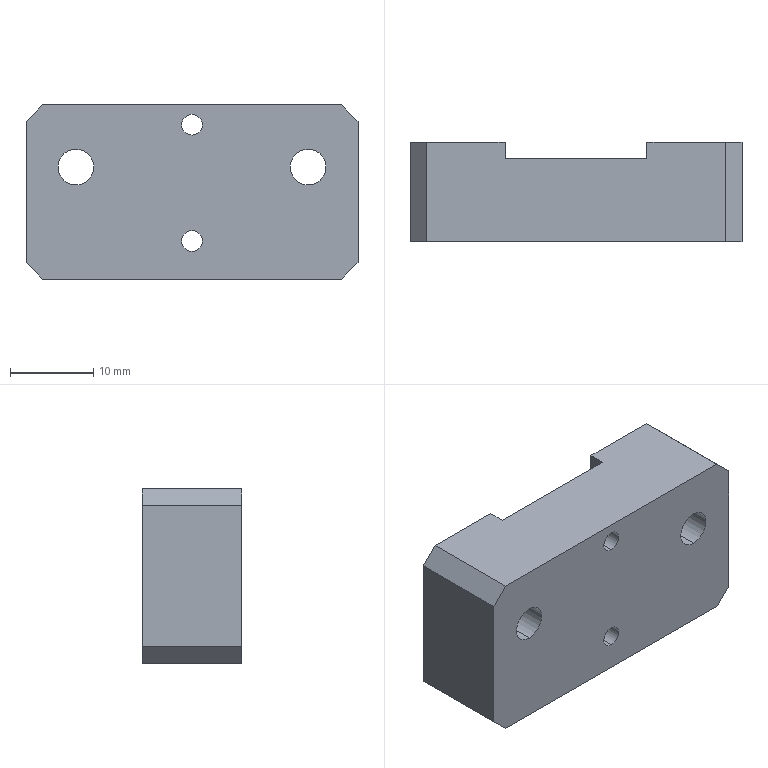Part | SolidWorks | features BaseBody 1 | 1 solid | 28 faces | box 40 x 12 x 21 mm | volume 8462 mm3 | plane 16 | cylinder 12 | commonest cylinder face diameters 2.5 x4 4.3 x4 8 x4
STEP:
#1=CARTESIAN_POINT('',(14.,7.,-1.));
#2=VERTEX_POINT('',#1);
#3=CARTESIAN_POINT('',(14.,7.,7.));
#4=VERTEX_POINT('',#3);
#5=CARTESIAN_POINT('',(14.,7.,3.));
#6=DIRECTION('',(0.,1.,0.));
#7=DIRECTION('',(0.,0.,1.));
#8=AXIS2_PLACEMENT_3D('',#5,#6,#7);
#9=CIRCLE('',#8,4.);
#10=EDGE_CURVE('',#2,#4,#9,.T.);
#11=ORIENTED_EDGE('',*,*,#10,.F.);
#12=CARTESIAN_POINT('',(14.,12.,-1.));
#13=VERTEX_POINT('',#12);
#14=CARTESIAN_POINT('',(14.,12.,-1.));
#15=DIRECTION('',(0.,1.,0.));
#16=VECTOR('',#15,1000.);
#17=LINE('',#14,#16);
#18=EDGE_CURVE('',#2,#13,#17,.T.);
#19=ORIENTED_EDGE('',*,*,#18,.T.);
#20=CARTESIAN_POINT('',(14.,12.,7.));
#21=VERTEX_POINT('',#20);
#22=CARTESIAN_POINT('',(14.,12.,3.));
#23=DIRECTION('',(0.,1.,0.));
#24=DIRECTION('',(0.,0.,1.));
#25=AXIS2_PLACEMENT_3D('',#22,#23,#24);
#26=CIRCLE('',#25,4.);
#27=EDGE_CURVE('',#13,#21,#26,.T.);
#28=ORIENTED_EDGE('',*,*,#27,.T.);
#29=CARTESIAN_POINT('',(14.,12.,7.));
#30=DIRECTION('',(0.,1.,0.));
#31=VECTOR('',#30,1000.);
#32=LINE('',#29,#31);
#33=EDGE_CURVE('',#4,#21,#32,.T.);
#34=ORIENTED_EDGE('',*,*,#33,.F.);
#35=EDGE_LOOP('',(#11,#19,#28,#34));
#36=FACE_OUTER_BOUND('',#35,.T.);
#37=CARTESIAN_POINT('',(14.,12.,3.));
#38=DIRECTION('',(0.,1.,0.));
#39=DIRECTION('',(0.,0.,1.));
#40=AXIS2_PLACEMENT_3D('',#37,#38,#39);
#41=CYLINDRICAL_SURFACE('',#40,4.);
#42=ADVANCED_FACE('',(#36),#41,.F.);
#43=CARTESIAN_POINT('',(14.,0.,0.85));
#44=VERTEX_POINT('',#43);
#45=CARTESIAN_POINT('',(14.,0.,5.15));
#46=VERTEX_POINT('',#45);
#47=CARTESIAN_POINT('',(14.,0.,3.));
#48=DIRECTION('',(0.,1.,0.));
#49=DIRECTION('',(0.,0.,1.));
#50=AXIS2_PLACEMENT_3D('',#47,#48,#49);
#51=CIRCLE('',#50,2.15);
#52=EDGE_CURVE('',#44,#46,#51,.T.);
#53=ORIENTED_EDGE('',*,*,#52,.F.);
#54=CARTESIAN_POINT('',(14.,7.,0.85));
#55=VERTEX_POINT('',#54);
#56=CARTESIAN_POINT('',(14.,12.,0.85));
#57=DIRECTION('',(0.,1.,0.));
#58=VECTOR('',#57,1000.);
#59=LINE('',#56,#58);
#60=EDGE_CURVE('',#44,#55,#59,.T.);
#61=ORIENTED_EDGE('',*,*,#60,.T.);
#62=CARTESIAN_POINT('',(14.,7.,5.15));
#63=VERTEX_POINT('',#62);
#64=CARTESIAN_POINT('',(14.,7.,3.));
#65=DIRECTION('',(0.,1.,0.));
#66=DIRECTION('',(0.,0.,1.));
#67=AXIS2_PLACEMENT_3D('',#64,#65,#66);
#68=CIRCLE('',#67,2.15);
#69=EDGE_CURVE('',#55,#63,#68,.T.);
#70=ORIENTED_EDGE('',*,*,#69,.T.);
#71=CARTESIAN_POINT('',(14.,12.,5.15));
#72=DIRECTION('',(0.,1.,0.));
#73=VECTOR('',#72,1000.);
#74=LINE('',#71,#73);
#75=EDGE_CURVE('',#46,#63,#74,.T.);
#76=ORIENTED_EDGE('',*,*,#75,.F.);
#77=EDGE_LOOP('',(#53,#61,#70,#76));
#78=FACE_OUTER_BOUND('',#77,.T.);
#79=CARTESIAN_POINT('',(14.,12.,3.));
#80=DIRECTION('',(0.,1.,0.));
#81=DIRECTION('',(0.,0.,1.));
#82=AXIS2_PLACEMENT_3D('',#79,#80,#81);
#83=CYLINDRICAL_SURFACE('',#82,2.15);
#84=ADVANCED_FACE('',(#78),#83,.F.);
#85=CARTESIAN_POINT('',(-14.,7.,-1.));
#86=VERTEX_POINT('',#85);
#87=CARTESIAN_POINT('',(-14.,7.,7.));
#88=VERTEX_POINT('',#87);
#89=CARTESIAN_POINT('',(-14.,7.,3.));
#90=DIRECTION('',(0.,1.,0.));
#91=DIRECTION('',(0.,0.,1.));
#92=AXIS2_PLACEMENT_3D('',#89,#90,#91);
#93=CIRCLE('',#92,4.);
#94=EDGE_CURVE('',#86,#88,#93,.T.);
#95=ORIENTED_EDGE('',*,*,#94,.F.);
#96=CARTESIAN_POINT('',(-14.,12.,-1.));
#97=VERTEX_POINT('',#96);
#98=CARTESIAN_POINT('',(-14.,12.,-1.));
#99=DIRECTION('',(0.,1.,0.));
#100=VECTOR('',#99,1000.);
#101=LINE('',#98,#100);
#102=EDGE_CURVE('',#86,#97,#101,.T.);
#103=ORIENTED_EDGE('',*,*,#102,.T.);
#104=CARTESIAN_POINT('',(-14.,12.,7.));
#105=VERTEX_POINT('',#104);
#106=CARTESIAN_POINT('',(-14.,12.,3.));
#107=DIRECTION('',(0.,1.,0.));
#108=DIRECTION('',(0.,0.,1.));
#109=AXIS2_PLACEMENT_3D('',#106,#107,#108);
#110=CIRCLE('',#109,4.);
#111=EDGE_CURVE('',#97,#105,#110,.T.);
#112=ORIENTED_EDGE('',*,*,#111,.T.);
#113=CARTESIAN_POINT('',(-14.,12.,7.));
#114=DIRECTION('',(0.,1.,0.));
#115=VECTOR('',#114,1000.);
#116=LINE('',#113,#115);
#117=EDGE_CURVE('',#88,#105,#116,.T.);
#118=ORIENTED_EDGE('',*,*,#117,.F.);
#119=EDGE_LOOP('',(#95,#103,#112,#118));
#120=FACE_OUTER_BOUND('',#119,.T.);
#121=CARTESIAN_POINT('',(-14.,12.,3.));
#122=DIRECTION('',(0.,1.,0.));
#123=DIRECTION('',(0.,0.,1.));
#124=AXIS2_PLACEMENT_3D('',#121,#122,#123);
#125=CYLINDRICAL_SURFACE('',#124,4.);
#126=ADVANCED_FACE('',(#120),#125,.F.);
#127=CARTESIAN_POINT('',(-14.,0.,0.85));
#128=VERTEX_POINT('',#127);
#129=CARTESIAN_POINT('',(-14.,0.,5.15));
#130=VERTEX_POINT('',#129);
#131=CARTESIAN_POINT('',(-14.,0.,3.));
#132=DIRECTION('',(0.,1.,0.));
#133=DIRECTION('',(0.,0.,1.));
#134=AXIS2_PLACEMENT_3D('',#131,#132,#133);
#135=CIRCLE('',#134,2.15);
#136=EDGE_CURVE('',#128,#130,#135,.T.);
#137=ORIENTED_EDGE('',*,*,#136,.F.);
#138=CARTESIAN_POINT('',(-14.,7.,0.85));
#139=VERTEX_POINT('',#138);
#140=CARTESIAN_POINT('',(-14.,12.,0.85));
#141=DIRECTION('',(0.,1.,0.));
#142=VECTOR('',#141,1000.);
#143=LINE('',#140,#142);
#144=EDGE_CURVE('',#128,#139,#143,.T.);
#145=ORIENTED_EDGE('',*,*,#144,.T.);
#146=CARTESIAN_POINT('',(-14.,7.,5.15));
#147=VERTEX_POINT('',#146);
#148=CARTESIAN_POINT('',(-14.,7.,3.));
#149=DIRECTION('',(0.,1.,0.));
#150=DIRECTION('',(0.,0.,1.));
#151=AXIS2_PLACEMENT_3D('',#148,#149,#150);
#152=CIRCLE('',#151,2.15);
#153=EDGE_CURVE('',#139,#147,#152,.T.);
#154=ORIENTED_EDGE('',*,*,#153,.T.);
#155=CARTESIAN_POINT('',(-14.,12.,5.15));
#156=DIRECTION('',(0.,1.,0.));
#157=VECTOR('',#156,1000.);
#158=LINE('',#155,#157);
#159=EDGE_CURVE('',#130,#147,#158,.T.);
#160=ORIENTED_EDGE('',*,*,#159,.F.);
#161=EDGE_LOOP('',(#137,#145,#154,#160));
#162=FACE_OUTER_BOUND('',#161,.T.);
#163=CARTESIAN_POINT('',(-14.,12.,3.));
#164=DIRECTION('',(0.,1.,0.));
#165=DIRECTION('',(0.,0.,1.));
#166=AXIS2_PLACEMENT_3D('',#163,#164,#165);
#167=CYLINDRICAL_SURFACE('',#166,2.15);
#168=ADVANCED_FACE('',(#162),#167,.F.);
#169=CARTESIAN_POINT('',(0.,0.,6.85));
#170=VERTEX_POINT('',#169);
#171=CARTESIAN_POINT('',(0.,0.,9.35));
#172=VERTEX_POINT('',#171);
#173=CARTESIAN_POINT('',(0.,0.,8.1));
#174=DIRECTION('',(0.,1.,0.));
#175=DIRECTION('',(0.,0.,1.));
#176=AXIS2_PLACEMENT_3D('',#173,#174,#175);
#177=CIRCLE('',#176,1.25);
#178=EDGE_CURVE('',#170,#172,#177,.T.);
#179=ORIENTED_EDGE('',*,*,#178,.F.);
#180=CARTESIAN_POINT('',(0.,10.,6.85));
#181=VERTEX_POINT('',#180);
#182=CARTESIAN_POINT('',(0.,12.,6.85));
#183=DIRECTION('',(0.,1.,0.));
#184=VECTOR('',#183,1000.);
#185=LINE('',#182,#184);
#186=EDGE_CURVE('',#170,#181,#185,.T.);
#187=ORIENTED_EDGE('',*,*,#186,.T.);
#188=CARTESIAN_POINT('',(0.,10.,9.35));
#189=VERTEX_POINT('',#188);
#190=CARTESIAN_POINT('',(0.,10.,8.1));
#191=DIRECTION('',(0.,1.,0.));
#192=DIRECTION('',(0.,0.,1.));
#193=AXIS2_PLACEMENT_3D('',#190,#191,#192);
#194=CIRCLE('',#193,1.25);
#195=EDGE_CURVE('',#181,#189,#194,.T.);
#196=ORIENTED_EDGE('',*,*,#195,.T.);
#197=CARTESIAN_POINT('',(0.,12.,9.35));
#198=DIRECTION('',(0.,1.,0.));
#199=VECTOR('',#198,1000.);
#200=LINE('',#197,#199);
#201=EDGE_CURVE('',#172,#189,#200,.T.);
#202=ORIENTED_EDGE('',*,*,#201,.F.);
#203=EDGE_LOOP('',(#179,#187,#196,#202));
#204=FACE_OUTER_BOUND('',#203,.T.);
#205=CARTESIAN_POINT('',(0.,12.,8.1));
#206=DIRECTION('',(0.,1.,0.));
#207=DIRECTION('',(0.,0.,1.));
#208=AXIS2_PLACEMENT_3D('',#205,#206,#207);
#209=CYLINDRICAL_SURFACE('',#208,1.25);
#210=ADVANCED_FACE('',(#204),#209,.F.);
#211=CARTESIAN_POINT('',(0.,0.,-7.15));
#212=VERTEX_POINT('',#211);
#213=CARTESIAN_POINT('',(0.,0.,-4.65));
#214=VERTEX_POINT('',#213);
#215=CARTESIAN_POINT('',(0.,0.,-5.9));
#216=DIRECTION('',(0.,1.,0.));
#217=DIRECTION('',(0.,0.,1.));
#218=AXIS2_PLACEMENT_3D('',#215,#216,#217);
#219=CIRCLE('',#218,1.25);
#220=EDGE_CURVE('',#212,#214,#219,.T.);
#221=ORIENTED_EDGE('',*,*,#220,.F.);
#222=CARTESIAN_POINT('',(0.,10.,-7.15));
#223=VERTEX_POINT('',#222);
#224=CARTESIAN_POINT('',(0.,12.,-7.15));
#225=DIRECTION('',(0.,1.,0.));
#226=VECTOR('',#225,1000.);
#227=LINE('',#224,#226);
#228=EDGE_CURVE('',#212,#223,#227,.T.);
#229=ORIENTED_EDGE('',*,*,#228,.T.);
#230=CARTESIAN_POINT('',(0.,10.,-4.65));
#231=VERTEX_POINT('',#230);
#232=CARTESIAN_POINT('',(0.,10.,-5.9));
#233=DIRECTION('',(0.,1.,0.));
#234=DIRECTION('',(0.,0.,1.));
#235=AXIS2_PLACEMENT_3D('',#232,#233,#234);
#236=CIRCLE('',#235,1.25);
#237=EDGE_CURVE('',#223,#231,#236,.T.);
#238=ORIENTED_EDGE('',*,*,#237,.T.);
#239=CARTESIAN_POINT('',(0.,12.,-4.65));
#240=DIRECTION('',(0.,1.,0.));
#241=VECTOR('',#240,1000.);
#242=LINE('',#239,#241);
#243=EDGE_CURVE('',#214,#231,#242,.T.);
#244=ORIENTED_EDGE('',*,*,#243,.F.);
#245=EDGE_LOOP('',(#221,#229,#238,#244));
#246=FACE_OUTER_BOUND('',#245,.T.);
#247=CARTESIAN_POINT('',(0.,12.,-5.9));
#248=DIRECTION('',(0.,1.,0.));
#249=DIRECTION('',(0.,0.,1.));
#250=AXIS2_PLACEMENT_3D('',#247,#248,#249);
#251=CYLINDRICAL_SURFACE('',#250,1.25);
#252=ADVANCED_FACE('',(#246),#251,.F.);
#253=CARTESIAN_POINT('',(-20.,12.,8.5));
#254=VERTEX_POINT('',#253);
#255=CARTESIAN_POINT('',(-18.,12.,10.5));
#256=VERTEX_POINT('',#255);
#257=CARTESIAN_POINT('',(-14.25,12.,14.25));
#258=DIRECTION('',(0.7071,0.,0.7071));
#259=VECTOR('',#258,1000.);
#260=LINE('',#257,#259);
#261=EDGE_CURVE('',#254,#256,#260,.T.);
#262=ORIENTED_EDGE('',*,*,#261,.F.);
#263=CARTESIAN_POINT('',(-20.,0.,8.5));
#264=VERTEX_POINT('',#263);
#265=CARTESIAN_POINT('',(-20.,12.,8.5));
#266=DIRECTION('',(0.,1.,0.));
#267=VECTOR('',#266,1000.);
#268=LINE('',#265,#267);
#269=EDGE_CURVE('',#264,#254,#268,.T.);
#270=ORIENTED_EDGE('',*,*,#269,.F.);
#271=CARTESIAN_POINT('',(-18.,0.,10.5));
#272=VERTEX_POINT('',#271);
#273=CARTESIAN_POINT('',(-18.,0.,10.5));
#274=DIRECTION('',(-0.7071,0.,-0.7071));
#275=VECTOR('',#274,1000.);
#276=LINE('',#273,#275);
#277=EDGE_CURVE('',#272,#264,#276,.T.);
#278=ORIENTED_EDGE('',*,*,#277,.F.);
#279=CARTESIAN_POINT('',(-18.,12.,10.5));
#280=DIRECTION('',(0.,-1.,0.));
#281=VECTOR('',#280,1000.);
#282=LINE('',#279,#281);
#283=EDGE_CURVE('',#256,#272,#282,.T.);
#284=ORIENTED_EDGE('',*,*,#283,.F.);
#285=EDGE_LOOP('',(#262,#270,#278,#284));
#286=FACE_OUTER_BOUND('',#285,.T.);
#287=CARTESIAN_POINT('',(-18.,12.,10.5));
#288=DIRECTION('',(0.7071,0.,-0.7071));
#289=DIRECTION('',(0.,-1.,0.));
#290=AXIS2_PLACEMENT_3D('',#287,#288,#289);
#291=PLANE('',#290);
#292=ADVANCED_FACE('',(#286),#291,.F.);
#293=CARTESIAN_POINT('',(18.,12.,10.5));
#294=VERTEX_POINT('',#293);
#295=CARTESIAN_POINT('',(20.,12.,8.5));
#296=VERTEX_POINT('',#295);
#297=CARTESIAN_POINT('',(14.25,12.,14.25));
#298=DIRECTION('',(0.7071,0.,-0.7071));
#299=VECTOR('',#298,1000.);
#300=LINE('',#297,#299);
#301=EDGE_CURVE('',#294,#296,#300,.T.);
#302=ORIENTED_EDGE('',*,*,#301,.F.);
#303=CARTESIAN_POINT('',(18.,0.,10.5));
#304=VERTEX_POINT('',#303);
#305=CARTESIAN_POINT('',(18.,12.,10.5));
#306=DIRECTION('',(0.,1.,0.));
#307=VECTOR('',#306,1000.);
#308=LINE('',#305,#307);
#309=EDGE_CURVE('',#304,#294,#308,.T.);
#310=ORIENTED_EDGE('',*,*,#309,.F.);
#311=CARTESIAN_POINT('',(20.,0.,8.5));
#312=VERTEX_POINT('',#311);
#313=CARTESIAN_POINT('',(20.,0.,8.5));
#314=DIRECTION('',(-0.7071,0.,0.7071));
#315=VECTOR('',#314,1000.);
#316=LINE('',#313,#315);
#317=EDGE_CURVE('',#312,#304,#316,.T.);
#318=ORIENTED_EDGE('',*,*,#317,.F.);
#319=CARTESIAN_POINT('',(20.,12.,8.5));
#320=DIRECTION('',(0.,-1.,0.));
#321=VECTOR('',#320,1000.);
#322=LINE('',#319,#321);
#323=EDGE_CURVE('',#296,#312,#322,.T.);
#324=ORIENTED_EDGE('',*,*,#323,.F.);
#325=EDGE_LOOP('',(#302,#310,#318,#324));
#326=FACE_OUTER_BOUND('',#325,.T.);
#327=CARTESIAN_POINT('',(20.,12.,8.5));
#328=DIRECTION('',(-0.7071,0.,-0.7071));
#329=DIRECTION('',(-0.7071,0.,0.7071));
#330=AXIS2_PLACEMENT_3D('',#327,#328,#329);
#331=PLANE('',#330);
#332=ADVANCED_FACE('',(#326),#331,.F.);
#333=CARTESIAN_POINT('',(20.,12.,-8.5));
#334=VERTEX_POINT('',#333);
#335=CARTESIAN_POINT('',(18.,12.,-10.5));
#336=VERTEX_POINT('',#335);
#337=CARTESIAN_POINT('',(14.25,12.,-14.25));
#338=DIRECTION('',(-0.7071,0.,-0.7071));
#339=VECTOR('',#338,1000.);
#340=LINE('',#337,#339);
#341=EDGE_CURVE('',#334,#336,#340,.T.);
#342=ORIENTED_EDGE('',*,*,#341,.F.);
#343=CARTESIAN_POINT('',(20.,0.,-8.5));
#344=VERTEX_POINT('',#343);
#345=CARTESIAN_POINT('',(20.,12.,-8.5));
#346=DIRECTION('',(0.,1.,0.));
#347=VECTOR('',#346,1000.);
#348=LINE('',#345,#347);
#349=EDGE_CURVE('',#344,#334,#348,.T.);
#350=ORIENTED_EDGE('',*,*,#349,.F.);
#351=CARTESIAN_POINT('',(18.,0.,-10.5));
#352=VERTEX_POINT('',#351);
#353=CARTESIAN_POINT('',(18.,0.,-10.5));
#354=DIRECTION('',(0.7071,0.,0.7071));
#355=VECTOR('',#354,1000.);
#356=LINE('',#353,#355);
#357=EDGE_CURVE('',#352,#344,#356,.T.);
#358=ORIENTED_EDGE('',*,*,#357,.F.);
#359=CARTESIAN_POINT('',(18.,12.,-10.5));
#360=DIRECTION('',(0.,-1.,0.));
#361=VECTOR('',#360,1000.);
#362=LINE('',#359,#361);
#363=EDGE_CURVE('',#336,#352,#362,.T.);
#364=ORIENTED_EDGE('',*,*,#363,.F.);
#365=EDGE_LOOP('',(#342,#350,#358,#364));
#366=FACE_OUTER_BOUND('',#365,.T.);
#367=CARTESIAN_POINT('',(18.,12.,-10.5));
#368=DIRECTION('',(-0.7071,0.,0.7071));
#369=DIRECTION('',(0.,1.,0.));
#370=AXIS2_PLACEMENT_3D('',#367,#368,#369);
#371=PLANE('',#370);
#372=ADVANCED_FACE('',(#366),#371,.F.);
#373=CARTESIAN_POINT('',(-18.,12.,-10.5));
#374=VERTEX_POINT('',#373);
#375=CARTESIAN_POINT('',(-20.,12.,-8.5));
#376=VERTEX_POINT('',#375);
#377=CARTESIAN_POINT('',(-14.25,12.,-14.25));
#378=DIRECTION('',(-0.7071,0.,0.7071));
#379=VECTOR('',#378,1000.);
#380=LINE('',#377,#379);
#381=EDGE_CURVE('',#374,#376,#380,.T.);
#382=ORIENTED_EDGE('',*,*,#381,.F.);
#383=CARTESIAN_POINT('',(-18.,0.,-10.5));
#384=VERTEX_POINT('',#383);
#385=CARTESIAN_POINT('',(-18.,12.,-10.5));
#386=DIRECTION('',(0.,1.,0.));
#387=VECTOR('',#386,1000.);
#388=LINE('',#385,#387);
#389=EDGE_CURVE('',#384,#374,#388,.T.);
#390=ORIENTED_EDGE('',*,*,#389,.F.);
#391=CARTESIAN_POINT('',(-20.,0.,-8.5));
#392=VERTEX_POINT('',#391);
#393=CARTESIAN_POINT('',(-20.,0.,-8.5));
#394=DIRECTION('',(0.7071,0.,-0.7071));
#395=VECTOR('',#394,1000.);
#396=LINE('',#393,#395);
#397=EDGE_CURVE('',#392,#384,#396,.T.);
#398=ORIENTED_EDGE('',*,*,#397,.F.);
#399=CARTESIAN_POINT('',(-20.,12.,-8.5));
#400=DIRECTION('',(0.,-1.,0.));
#401=VECTOR('',#400,1000.);
#402=LINE('',#399,#401);
#403=EDGE_CURVE('',#376,#392,#402,.T.);
#404=ORIENTED_EDGE('',*,*,#403,.F.);
#405=EDGE_LOOP('',(#382,#390,#398,#404));
#406=FACE_OUTER_BOUND('',#405,.T.);
#407=CARTESIAN_POINT('',(-20.,12.,-8.5));
#408=DIRECTION('',(0.7071,0.,0.7071));
#409=DIRECTION('',(0.,-1.,0.));
#410=AXIS2_PLACEMENT_3D('',#407,#408,#409);
#411=PLANE('',#410);
#412=ADVANCED_FACE('',(#406),#411,.F.);
#413=CARTESIAN_POINT('',(14.,7.,3.));
#414=DIRECTION('',(0.,1.,0.));
#415=DIRECTION('',(0.,0.,1.));
#416=AXIS2_PLACEMENT_3D('',#413,#414,#415);
#417=CIRCLE('',#416,2.15);
#418=EDGE_CURVE('',#63,#55,#417,.T.);
#419=ORIENTED_EDGE('',*,*,#418,.F.);
#420=ORIENTED_EDGE('',*,*,#69,.F.);
#421=EDGE_LOOP('',(#419,#420));
#422=FACE_BOUND('',#421,.T.);
#423=CARTESIAN_POINT('',(14.,7.,3.));
#424=DIRECTION('',(0.,1.,0.));
#425=DIRECTION('',(0.,0.,1.));
#426=AXIS2_PLACEMENT_3D('',#423,#424,#425);
#427=CIRCLE('',#426,4.);
#428=EDGE_CURVE('',#4,#2,#427,.T.);
#429=ORIENTED_EDGE('',*,*,#428,.T.);
#430=ORIENTED_EDGE('',*,*,#10,.T.);
#431=EDGE_LOOP('',(#429,#430));
#432=FACE_OUTER_BOUND('',#431,.T.);
#433=CARTESIAN_POINT('',(16.15,7.,3.));
#434=DIRECTION('',(0.,-1.,0.));
#435=DIRECTION('',(0.,0.,-1.));
#436=AXIS2_PLACEMENT_3D('',#433,#434,#435);
#437=PLANE('',#436);
#438=ADVANCED_FACE('',(#422,#432),#437,.F.);
#439=CARTESIAN_POINT('',(-14.,7.,3.));
#440=DIRECTION('',(0.,1.,0.));
#441=DIRECTION('',(0.,0.,1.));
#442=AXIS2_PLACEMENT_3D('',#439,#440,#441);
#443=CIRCLE('',#442,2.15);
#444=EDGE_CURVE('',#147,#139,#443,.T.);
#445=ORIENTED_EDGE('',*,*,#444,.F.);
#446=ORIENTED_EDGE('',*,*,#153,.F.);
#447=EDGE_LOOP('',(#445,#446));
#448=FACE_BOUND('',#447,.T.);
#449=CARTESIAN_POINT('',(-14.,7.,3.));
#450=DIRECTION('',(0.,1.,0.));
#451=DIRECTION('',(0.,0.,1.));
#452=AXIS2_PLACEMENT_3D('',#449,#450,#451);
#453=CIRCLE('',#452,4.);
#454=EDGE_CURVE('',#88,#86,#453,.T.);
#455=ORIENTED_EDGE('',*,*,#454,.T.);
#456=ORIENTED_EDGE('',*,*,#94,.T.);
#457=EDGE_LOOP('',(#455,#456));
#458=FACE_OUTER_BOUND('',#457,.T.);
#459=CARTESIAN_POINT('',(-11.85,7.,3.));
#460=DIRECTION('',(0.,-1.,0.));
#461=DIRECTION('',(0.,0.,-1.));
#462=AXIS2_PLACEMENT_3D('',#459,#460,#461);
#463=PLANE('',#462);
#464=ADVANCED_FACE('',(#448,#458),#463,.F.);
#465=CARTESIAN_POINT('',(-8.55,12.,-10.5));
#466=VERTEX_POINT('',#465);
#467=CARTESIAN_POINT('',(-8.55,12.,10.5));
#468=VERTEX_POINT('',#467);
#469=CARTESIAN_POINT('',(-8.55,12.,0.));
#470=DIRECTION('',(0.,0.,1.));
#471=VECTOR('',#470,1000.);
#472=LINE('',#469,#471);
#473=EDGE_CURVE('',#466,#468,#472,.T.);
#474=ORIENTED_EDGE('',*,*,#473,.T.);
#475=CARTESIAN_POINT('',(-8.55,10.,10.5));
#476=VERTEX_POINT('',#475);
#477=CARTESIAN_POINT('',(-8.55,12.,10.5));
#478=DIRECTION('',(0.,1.,0.));
#479=VECTOR('',#478,1000.);
#480=LINE('',#477,#479);
#481=EDGE_CURVE('',#476,#468,#480,.T.);
#482=ORIENTED_EDGE('',*,*,#481,.F.);
#483=CARTESIAN_POINT('',(-8.55,10.,-10.5));
#484=VERTEX_POINT('',#483);
#485=CARTESIAN_POINT('',(-8.55,10.,-15.));
#486=DIRECTION('',(0.,0.,1.));
#487=VECTOR('',#486,1000.);
#488=LINE('',#485,#487);
#489=EDGE_CURVE('',#484,#476,#488,.T.);
#490=ORIENTED_EDGE('',*,*,#489,.F.);
#491=CARTESIAN_POINT('',(-8.55,12.,-10.5));
#492=DIRECTION('',(0.,-1.,0.));
#493=VECTOR('',#492,1000.);
#494=LINE('',#491,#493);
#495=EDGE_CURVE('',#466,#484,#494,.T.);
#496=ORIENTED_EDGE('',*,*,#495,.F.);
#497=EDGE_LOOP('',(#474,#482,#490,#496));
#498=FACE_OUTER_BOUND('',#497,.T.);
#499=CARTESIAN_POINT('',(-8.55,10.,-15.));
#500=DIRECTION('',(-1.,0.,0.));
#501=DIRECTION('',(0.,1.,0.));
#502=AXIS2_PLACEMENT_3D('',#499,#500,#501);
#503=PLANE('',#502);
#504=ADVANCED_FACE('',(#498),#503,.F.);
#505=CARTESIAN_POINT('',(8.55,10.,10.5));
#506=VERTEX_POINT('',#505);
#507=CARTESIAN_POINT('',(8.55,10.,-10.5));
#508=VERTEX_POINT('',#507);
#509=CARTESIAN_POINT('',(8.55,10.,-15.));
#510=DIRECTION('',(0.,0.,-1.));
#511=VECTOR('',#510,1000.);
#512=LINE('',#509,#511);
#513=EDGE_CURVE('',#506,#508,#512,.T.);
#514=ORIENTED_EDGE('',*,*,#513,.F.);
#515=CARTESIAN_POINT('',(8.55,12.,10.5));
#516=VERTEX_POINT('',#515);
#517=CARTESIAN_POINT('',(8.55,12.,10.5));
#518=DIRECTION('',(0.,-1.,0.));
#519=VECTOR('',#518,1000.);
#520=LINE('',#517,#519);
#521=EDGE_CURVE('',#516,#506,#520,.T.);
#522=ORIENTED_EDGE('',*,*,#521,.F.);
#523=CARTESIAN_POINT('',(8.55,12.,-10.5));
#524=VERTEX_POINT('',#523);
#525=CARTESIAN_POINT('',(8.55,12.,0.));
#526=DIRECTION('',(0.,0.,-1.));
#527=VECTOR('',#526,1000.);
#528=LINE('',#525,#527);
#529=EDGE_CURVE('',#516,#524,#528,.T.);
#530=ORIENTED_EDGE('',*,*,#529,.T.);
#531=CARTESIAN_POINT('',(8.55,12.,-10.5));
#532=DIRECTION('',(0.,1.,0.));
#533=VECTOR('',#532,1000.);
#534=LINE('',#531,#533);
#535=EDGE_CURVE('',#508,#524,#534,.T.);
#536=ORIENTED_EDGE('',*,*,#535,.F.);
#537=EDGE_LOOP('',(#514,#522,#530,#536));
#538=FACE_OUTER_BOUND('',#537,.T.);
#539=CARTESIAN_POINT('',(8.55,10.,-15.));
#540=DIRECTION('',(1.,0.,0.));
#541=DIRECTION('',(0.,0.,-1.));
#542=AXIS2_PLACEMENT_3D('',#539,#540,#541);
#543=PLANE('',#542);
#544=ADVANCED_FACE('',(#538),#543,.F.);
#545=CARTESIAN_POINT('',(0.,10.,-5.9));
#546=DIRECTION('',(0.,1.,0.));
#547=DIRECTION('',(0.,0.,1.));
#548=AXIS2_PLACEMENT_3D('',#545,#546,#547);
#549=CIRCLE('',#548,1.25);
#550=EDGE_CURVE('',#231,#223,#549,.T.);
#551=ORIENTED_EDGE('',*,*,#550,.F.);
#552=ORIENTED_EDGE('',*,*,#237,.F.);
#553=EDGE_LOOP('',(#551,#552));
#554=FACE_BOUND('',#553,.T.);
#555=CARTESIAN_POINT('',(0.,10.,8.1));
#556=DIRECTION('',(0.,1.,0.));
#557=DIRECTION('',(0.,0.,1.));
#558=AXIS2_PLACEMENT_3D('',#555,#556,#557);
#559=CIRCLE('',#558,1.25);
#560=EDGE_CURVE('',#189,#181,#559,.T.);
#561=ORIENTED_EDGE('',*,*,#560,.F.);
#562=ORIENTED_EDGE('',*,*,#195,.F.);
#563=EDGE_LOOP('',(#561,#562));
#564=FACE_BOUND('',#563,.T.);
#565=CARTESIAN_POINT('',(-20.,10.,-10.5));
#566=DIRECTION('',(-1.,0.,0.));
#567=VECTOR('',#566,1000.);
#568=LINE('',#565,#567);
#569=EDGE_CURVE('',#508,#484,#568,.T.);
#570=ORIENTED_EDGE('',*,*,#569,.T.);
#571=ORIENTED_EDGE('',*,*,#489,.T.);
#572=CARTESIAN_POINT('',(-20.,10.,10.5));
#573=DIRECTION('',(1.,0.,0.));
#574=VECTOR('',#573,1000.);
#575=LINE('',#572,#574);
#576=EDGE_CURVE('',#476,#506,#575,.T.);
#577=ORIENTED_EDGE('',*,*,#576,.T.);
#578=ORIENTED_EDGE('',*,*,#513,.T.);
#579=EDGE_LOOP('',(#570,#571,#577,#578));
#580=FACE_OUTER_BOUND('',#579,.T.);
#581=CARTESIAN_POINT('',(0.,10.,0.));
#582=DIRECTION('',(0.,1.,0.));
#583=DIRECTION('',(1.,0.,0.));
#584=AXIS2_PLACEMENT_3D('',#581,#582,#583);
#585=PLANE('',#584);
#586=ADVANCED_FACE('',(#554,#564,#580),#585,.T.);
#587=CARTESIAN_POINT('',(0.,0.,-5.9));
#588=DIRECTION('',(0.,1.,0.));
#589=DIRECTION('',(0.,0.,1.));
#590=AXIS2_PLACEMENT_3D('',#587,#588,#589);
#591=CIRCLE('',#590,1.25);
#592=EDGE_CURVE('',#214,#212,#591,.T.);
#593=ORIENTED_EDGE('',*,*,#592,.T.);
#594=ORIENTED_EDGE('',*,*,#220,.T.);
#595=EDGE_LOOP('',(#593,#594));
#596=FACE_BOUND('',#595,.T.);
#597=CARTESIAN_POINT('',(0.,0.,8.1));
#598=DIRECTION('',(0.,1.,0.));
#599=DIRECTION('',(0.,0.,1.));
#600=AXIS2_PLACEMENT_3D('',#597,#598,#599);
#601=CIRCLE('',#600,1.25);
#602=EDGE_CURVE('',#172,#170,#601,.T.);
#603=ORIENTED_EDGE('',*,*,#602,.T.);
#604=ORIENTED_EDGE('',*,*,#178,.T.);
#605=EDGE_LOOP('',(#603,#604));
#606=FACE_BOUND('',#605,.T.);
#607=CARTESIAN_POINT('',(-14.,0.,3.));
#608=DIRECTION('',(0.,1.,0.));
#609=DIRECTION('',(0.,0.,1.));
#610=AXIS2_PLACEMENT_3D('',#607,#608,#609);
#611=CIRCLE('',#610,2.15);
#612=EDGE_CURVE('',#130,#128,#611,.T.);
#613=ORIENTED_EDGE('',*,*,#612,.T.);
#614=ORIENTED_EDGE('',*,*,#136,.T.);
#615=EDGE_LOOP('',(#613,#614));
#616=FACE_BOUND('',#615,.T.);
#617=CARTESIAN_POINT('',(14.,0.,3.));
#618=DIRECTION('',(0.,1.,0.));
#619=DIRECTION('',(0.,0.,1.));
#620=AXIS2_PLACEMENT_3D('',#617,#618,#619);
#621=CIRCLE('',#620,2.15);
#622=EDGE_CURVE('',#46,#44,#621,.T.);
#623=ORIENTED_EDGE('',*,*,#622,.T.);
#624=ORIENTED_EDGE('',*,*,#52,.T.);
#625=EDGE_LOOP('',(#623,#624));
#626=FACE_BOUND('',#625,.T.);
#627=CARTESIAN_POINT('',(-20.,0.,-10.5));
#628=DIRECTION('',(0.,0.,1.));
#629=VECTOR('',#628,1000.);
#630=LINE('',#627,#629);
#631=EDGE_CURVE('',#392,#264,#630,.T.);
#632=ORIENTED_EDGE('',*,*,#631,.F.);
#633=ORIENTED_EDGE('',*,*,#397,.T.);
#634=CARTESIAN_POINT('',(-20.,0.,-10.5));
#635=DIRECTION('',(-1.,0.,0.));
#636=VECTOR('',#635,1000.);
#637=LINE('',#634,#636);
#638=EDGE_CURVE('',#352,#384,#637,.T.);
#639=ORIENTED_EDGE('',*,*,#638,.F.);
#640=ORIENTED_EDGE('',*,*,#357,.T.);
#641=CARTESIAN_POINT('',(20.,0.,-10.5));
#642=DIRECTION('',(0.,0.,-1.));
#643=VECTOR('',#642,1000.);
#644=LINE('',#641,#643);
#645=EDGE_CURVE('',#312,#344,#644,.T.);
#646=ORIENTED_EDGE('',*,*,#645,.F.);
#647=ORIENTED_EDGE('',*,*,#317,.T.);
#648=CARTESIAN_POINT('',(-20.,0.,10.5));
#649=DIRECTION('',(1.,0.,0.));
#650=VECTOR('',#649,1000.);
#651=LINE('',#648,#650);
#652=EDGE_CURVE('',#272,#304,#651,.T.);
#653=ORIENTED_EDGE('',*,*,#652,.F.);
#654=ORIENTED_EDGE('',*,*,#277,.T.);
#655=EDGE_LOOP('',(#632,#633,#639,#640,#646,#647,#653,#654));
#656=FACE_OUTER_BOUND('',#655,.T.);
#657=CARTESIAN_POINT('',(0.,0.,0.));
#658=DIRECTION('',(0.,1.,0.));
#659=DIRECTION('',(1.,0.,0.));
#660=AXIS2_PLACEMENT_3D('',#657,#658,#659);
#661=PLANE('',#660);
#662=ADVANCED_FACE('',(#596,#606,#616,#626,#656),#661,.F.);
#663=CARTESIAN_POINT('',(-14.,12.,3.));
#664=DIRECTION('',(0.,1.,0.));
#665=DIRECTION('',(0.,0.,1.));
#666=AXIS2_PLACEMENT_3D('',#663,#664,#665);
#667=CIRCLE('',#666,4.);
#668=EDGE_CURVE('',#105,#97,#667,.T.);
#669=ORIENTED_EDGE('',*,*,#668,.F.);
#670=ORIENTED_EDGE('',*,*,#111,.F.);
#671=EDGE_LOOP('',(#669,#670));
#672=FACE_BOUND('',#671,.T.);
#673=CARTESIAN_POINT('',(-20.,12.,-10.5));
#674=DIRECTION('',(-1.,0.,0.));
#675=VECTOR('',#674,1000.);
#676=LINE('',#673,#675);
#677=EDGE_CURVE('',#466,#374,#676,.T.);
#678=ORIENTED_EDGE('',*,*,#677,.T.);
#679=ORIENTED_EDGE('',*,*,#381,.T.);
#680=CARTESIAN_POINT('',(-20.,12.,-10.5));
#681=DIRECTION('',(0.,0.,1.));
#682=VECTOR('',#681,1000.);
#683=LINE('',#680,#682);
#684=EDGE_CURVE('',#376,#254,#683,.T.);
#685=ORIENTED_EDGE('',*,*,#684,.T.);
#686=ORIENTED_EDGE('',*,*,#261,.T.);
#687=CARTESIAN_POINT('',(-20.,12.,10.5));
#688=DIRECTION('',(1.,0.,0.));
#689=VECTOR('',#688,1000.);
#690=LINE('',#687,#689);
#691=EDGE_CURVE('',#256,#468,#690,.T.);
#692=ORIENTED_EDGE('',*,*,#691,.T.);
#693=ORIENTED_EDGE('',*,*,#473,.F.);
#694=EDGE_LOOP('',(#678,#679,#685,#686,#692,#693));
#695=FACE_OUTER_BOUND('',#694,.T.);
#696=CARTESIAN_POINT('',(0.,12.,0.));
#697=DIRECTION('',(0.,1.,0.));
#698=DIRECTION('',(1.,0.,0.));
#699=AXIS2_PLACEMENT_3D('',#696,#697,#698);
#700=PLANE('',#699);
#701=ADVANCED_FACE('',(#672,#695),#700,.T.);
#702=ORIENTED_EDGE('',*,*,#652,.T.);
#703=ORIENTED_EDGE('',*,*,#309,.T.);
#704=CARTESIAN_POINT('',(-20.,12.,10.5));
#705=DIRECTION('',(1.,0.,0.));
#706=VECTOR('',#705,1000.);
#707=LINE('',#704,#706);
#708=EDGE_CURVE('',#516,#294,#707,.T.);
#709=ORIENTED_EDGE('',*,*,#708,.F.);
#710=ORIENTED_EDGE('',*,*,#521,.T.);
#711=ORIENTED_EDGE('',*,*,#576,.F.);
#712=ORIENTED_EDGE('',*,*,#481,.T.);
#713=ORIENTED_EDGE('',*,*,#691,.F.);
#714=ORIENTED_EDGE('',*,*,#283,.T.);
#715=EDGE_LOOP('',(#702,#703,#709,#710,#711,#712,#713,#714));
#716=FACE_OUTER_BOUND('',#715,.T.);
#717=CARTESIAN_POINT('',(-20.,12.,10.5));
#718=DIRECTION('',(0.,0.,-1.));
#719=DIRECTION('',(0.,-1.,0.));
#720=AXIS2_PLACEMENT_3D('',#717,#718,#719);
#721=PLANE('',#720);
#722=ADVANCED_FACE('',(#716),#721,.F.);
#723=ORIENTED_EDGE('',*,*,#684,.F.);
#724=ORIENTED_EDGE('',*,*,#403,.T.);
#725=ORIENTED_EDGE('',*,*,#631,.T.);
#726=ORIENTED_EDGE('',*,*,#269,.T.);
#727=EDGE_LOOP('',(#723,#724,#725,#726));
#728=FACE_OUTER_BOUND('',#727,.T.);
#729=CARTESIAN_POINT('',(-20.,12.,-10.5));
#730=DIRECTION('',(1.,0.,0.));
#731=DIRECTION('',(0.,0.,-1.));
#732=AXIS2_PLACEMENT_3D('',#729,#730,#731);
#733=PLANE('',#732);
#734=ADVANCED_FACE('',(#728),#733,.F.);
#735=ORIENTED_EDGE('',*,*,#638,.T.);
#736=ORIENTED_EDGE('',*,*,#389,.T.);
#737=ORIENTED_EDGE('',*,*,#677,.F.);
#738=ORIENTED_EDGE('',*,*,#495,.T.);
#739=ORIENTED_EDGE('',*,*,#569,.F.);
#740=ORIENTED_EDGE('',*,*,#535,.T.);
#741=CARTESIAN_POINT('',(-20.,12.,-10.5));
#742=DIRECTION('',(-1.,0.,0.));
#743=VECTOR('',#742,1000.);
#744=LINE('',#741,#743);
#745=EDGE_CURVE('',#336,#524,#744,.T.);
#746=ORIENTED_EDGE('',*,*,#745,.F.);
#747=ORIENTED_EDGE('',*,*,#363,.T.);
#748=EDGE_LOOP('',(#735,#736,#737,#738,#739,#740,#746,#747));
#749=FACE_OUTER_BOUND('',#748,.T.);
#750=CARTESIAN_POINT('',(-20.,12.,-10.5));
#751=DIRECTION('',(0.,0.,1.));
#752=DIRECTION('',(1.,0.,0.));
#753=AXIS2_PLACEMENT_3D('',#750,#751,#752);
#754=PLANE('',#753);
#755=ADVANCED_FACE('',(#749),#754,.F.);
#756=ORIENTED_EDGE('',*,*,#645,.T.);
#757=ORIENTED_EDGE('',*,*,#349,.T.);
#758=CARTESIAN_POINT('',(20.,12.,-10.5));
#759=DIRECTION('',(0.,0.,-1.));
#760=VECTOR('',#759,1000.);
#761=LINE('',#758,#760);
#762=EDGE_CURVE('',#296,#334,#761,.T.);
#763=ORIENTED_EDGE('',*,*,#762,.F.);
#764=ORIENTED_EDGE('',*,*,#323,.T.);
#765=EDGE_LOOP('',(#756,#757,#763,#764));
#766=FACE_OUTER_BOUND('',#765,.T.);
#767=CARTESIAN_POINT('',(20.,12.,-10.5));
#768=DIRECTION('',(-1.,0.,0.));
#769=DIRECTION('',(0.,0.,1.));
#770=AXIS2_PLACEMENT_3D('',#767,#768,#769);
#771=PLANE('',#770);
#772=ADVANCED_FACE('',(#766),#771,.F.);
#773=CARTESIAN_POINT('',(14.,12.,3.));
#774=DIRECTION('',(0.,1.,0.));
#775=DIRECTION('',(0.,0.,1.));
#776=AXIS2_PLACEMENT_3D('',#773,#774,#775);
#777=CIRCLE('',#776,4.);
#778=EDGE_CURVE('',#21,#13,#777,.T.);
#779=ORIENTED_EDGE('',*,*,#778,.F.);
#780=ORIENTED_EDGE('',*,*,#27,.F.);
#781=EDGE_LOOP('',(#779,#780));
#782=FACE_BOUND('',#781,.T.);
#783=ORIENTED_EDGE('',*,*,#762,.T.);
#784=ORIENTED_EDGE('',*,*,#341,.T.);
#785=ORIENTED_EDGE('',*,*,#745,.T.);
#786=ORIENTED_EDGE('',*,*,#529,.F.);
#787=ORIENTED_EDGE('',*,*,#708,.T.);
#788=ORIENTED_EDGE('',*,*,#301,.T.);
#789=EDGE_LOOP('',(#783,#784,#785,#786,#787,#788));
#790=FACE_OUTER_BOUND('',#789,.T.);
#791=CARTESIAN_POINT('',(0.,12.,0.));
#792=DIRECTION('',(0.,1.,0.));
#793=DIRECTION('',(1.,0.,0.));
#794=AXIS2_PLACEMENT_3D('',#791,#792,#793);
#795=PLANE('',#794);
#796=ADVANCED_FACE('',(#782,#790),#795,.T.);
#797=ORIENTED_EDGE('',*,*,#228,.F.);
#798=ORIENTED_EDGE('',*,*,#592,.F.);
#799=ORIENTED_EDGE('',*,*,#243,.T.);
#800=ORIENTED_EDGE('',*,*,#550,.T.);
#801=EDGE_LOOP('',(#797,#798,#799,#800));
#802=FACE_OUTER_BOUND('',#801,.T.);
#803=CARTESIAN_POINT('',(0.,12.,-5.9));
#804=DIRECTION('',(0.,1.,0.));
#805=DIRECTION('',(0.,0.,1.));
#806=AXIS2_PLACEMENT_3D('',#803,#804,#805);
#807=CYLINDRICAL_SURFACE('',#806,1.25);
#808=ADVANCED_FACE('',(#802),#807,.F.);
#809=ORIENTED_EDGE('',*,*,#186,.F.);
#810=ORIENTED_EDGE('',*,*,#602,.F.);
#811=ORIENTED_EDGE('',*,*,#201,.T.);
#812=ORIENTED_EDGE('',*,*,#560,.T.);
#813=EDGE_LOOP('',(#809,#810,#811,#812));
#814=FACE_OUTER_BOUND('',#813,.T.);
#815=CARTESIAN_POINT('',(0.,12.,8.1));
#816=DIRECTION('',(0.,1.,0.));
#817=DIRECTION('',(0.,0.,1.));
#818=AXIS2_PLACEMENT_3D('',#815,#816,#817);
#819=CYLINDRICAL_SURFACE('',#818,1.25);
#820=ADVANCED_FACE('',(#814),#819,.F.);
#821=ORIENTED_EDGE('',*,*,#144,.F.);
#822=ORIENTED_EDGE('',*,*,#612,.F.);
#823=ORIENTED_EDGE('',*,*,#159,.T.);
#824=ORIENTED_EDGE('',*,*,#444,.T.);
#825=EDGE_LOOP('',(#821,#822,#823,#824));
#826=FACE_OUTER_BOUND('',#825,.T.);
#827=CARTESIAN_POINT('',(-14.,12.,3.));
#828=DIRECTION('',(0.,1.,0.));
#829=DIRECTION('',(0.,0.,1.));
#830=AXIS2_PLACEMENT_3D('',#827,#828,#829);
#831=CYLINDRICAL_SURFACE('',#830,2.15);
#832=ADVANCED_FACE('',(#826),#831,.F.);
#833=ORIENTED_EDGE('',*,*,#102,.F.);
#834=ORIENTED_EDGE('',*,*,#454,.F.);
#835=ORIENTED_EDGE('',*,*,#117,.T.);
#836=ORIENTED_EDGE('',*,*,#668,.T.);
#837=EDGE_LOOP('',(#833,#834,#835,#836));
#838=FACE_OUTER_BOUND('',#837,.T.);
#839=CARTESIAN_POINT('',(-14.,12.,3.));
#840=DIRECTION('',(0.,1.,0.));
#841=DIRECTION('',(0.,0.,1.));
#842=AXIS2_PLACEMENT_3D('',#839,#840,#841);
#843=CYLINDRICAL_SURFACE('',#842,4.);
#844=ADVANCED_FACE('',(#838),#843,.F.);
#845=ORIENTED_EDGE('',*,*,#60,.F.);
#846=ORIENTED_EDGE('',*,*,#622,.F.);
#847=ORIENTED_EDGE('',*,*,#75,.T.);
#848=ORIENTED_EDGE('',*,*,#418,.T.);
#849=EDGE_LOOP('',(#845,#846,#847,#848));
#850=FACE_OUTER_BOUND('',#849,.T.);
#851=CARTESIAN_POINT('',(14.,12.,3.));
#852=DIRECTION('',(0.,1.,0.));
#853=DIRECTION('',(0.,0.,1.));
#854=AXIS2_PLACEMENT_3D('',#851,#852,#853);
#855=CYLINDRICAL_SURFACE('',#854,2.15);
#856=ADVANCED_FACE('',(#850),#855,.F.);
#857=ORIENTED_EDGE('',*,*,#18,.F.);
#858=ORIENTED_EDGE('',*,*,#428,.F.);
#859=ORIENTED_EDGE('',*,*,#33,.T.);
#860=ORIENTED_EDGE('',*,*,#778,.T.);
#861=EDGE_LOOP('',(#857,#858,#859,#860));
#862=FACE_OUTER_BOUND('',#861,.T.);
#863=CARTESIAN_POINT('',(14.,12.,3.));
#864=DIRECTION('',(0.,1.,0.));
#865=DIRECTION('',(0.,0.,1.));
#866=AXIS2_PLACEMENT_3D('',#863,#864,#865);
#867=CYLINDRICAL_SURFACE('',#866,4.);
#868=ADVANCED_FACE('',(#862),#867,.F.);
#869=CLOSED_SHELL('',(#42,#84,#126,#168,#210,#252,#292,#332,#372,#412,#438,#464,#504,#544,#586,#662,#701,#722,#734,#755,#772,#796,#808,#820,#832,#844,#856,#868));
#870=MANIFOLD_SOLID_BREP('',#869);
#871=CARTESIAN_POINT('',(0.,0.,0.));
#872=DIRECTION('',(0.,0.,1.));
#873=DIRECTION('',(1.,0.,0.));
#874=AXIS2_PLACEMENT_3D('',#871,#872,#873);
#875=(LENGTH_UNIT()NAMED_UNIT(*)SI_UNIT(.MILLI.,.METRE.));
#876=UNCERTAINTY_MEASURE_WITH_UNIT(LENGTH_MEASURE(0.00001),#875,'','');
#877=(NAMED_UNIT(*)PLANE_ANGLE_UNIT()SI_UNIT($,.RADIAN.));
#878=(NAMED_UNIT(*)SI_UNIT($,.STERADIAN.)SOLID_ANGLE_UNIT());
#879=(GEOMETRIC_REPRESENTATION_CONTEXT(3)GLOBAL_UNCERTAINTY_ASSIGNED_CONTEXT((#876))GLOBAL_UNIT_ASSIGNED_CONTEXT((#875,#877,#878))REPRESENTATION_CONTEXT('',''));
#880=ADVANCED_BREP_SHAPE_REPRESENTATION('',(#870,#874),#879);